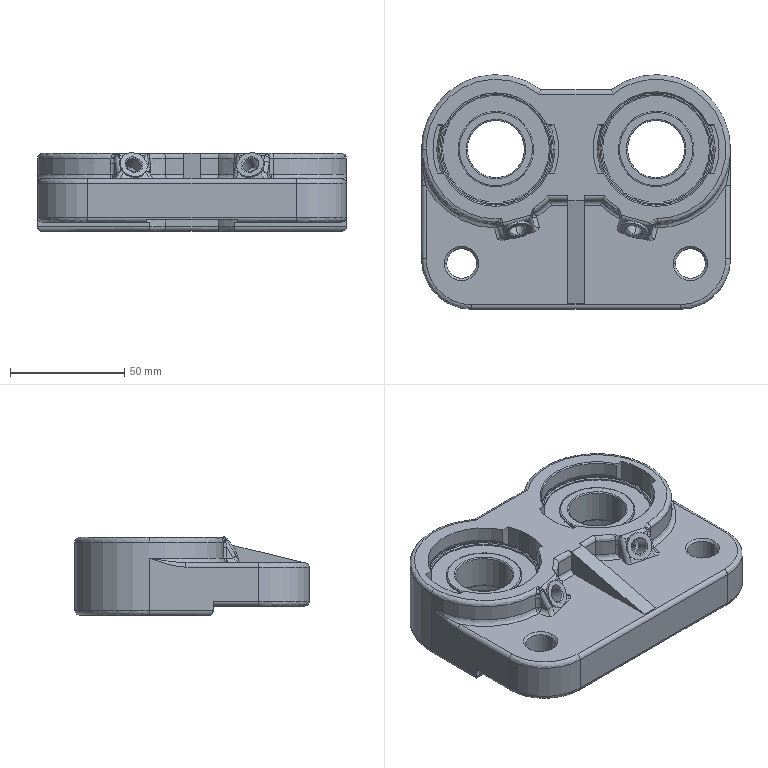Part | SolidWorks | features LayoutProfileFeature 1 | 3 solids | 290 faces | box 135 x 102.5 x 34.325 mm | volume 251519 mm3 | cylinder 106 | spline 89 | plane 68 | cone 27 | commonest cylinder face diameters 4 x37 33 x8 46.79 x8 49.143 x8 65 x7 54 x6